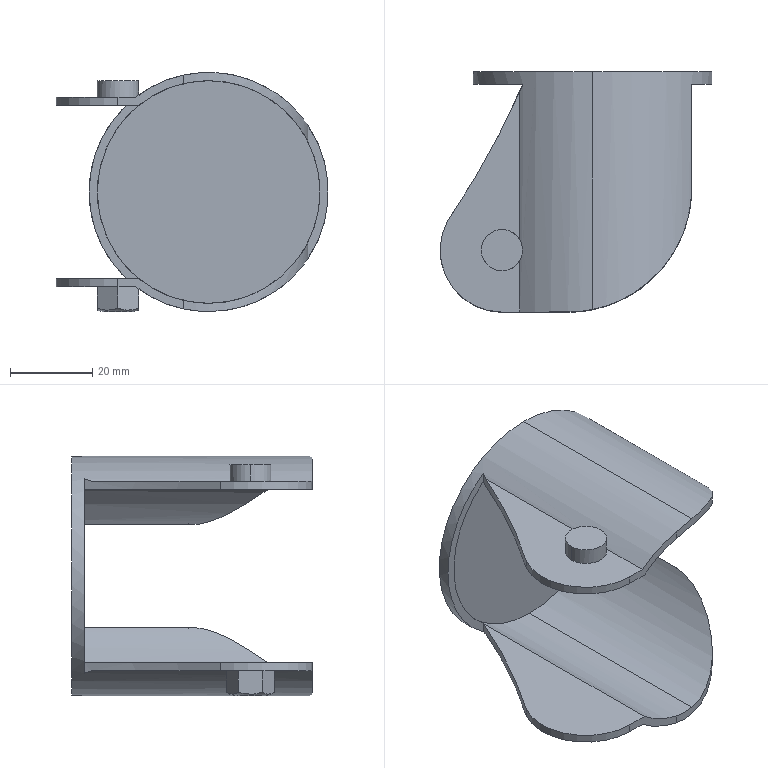Part | SolidWorks | features RefAxis 15, ICE 6, 3DProfileFeature 5, Revolution 2 | 1 solid | 36 faces | box 66 x 58.3 x 58 mm | volume 18491 mm3 | plane 20 | cylinder 14 | torus 2 | commonest cylinder face diameters 10 x2 12 x2 30 x2 54 x2 58 x2 60 x2
STEP:
#1=CARTESIAN_POINT('',(-17.,-56.613,-28.187));
#2=VERTEX_POINT('',#1);
#3=CARTESIAN_POINT('',(-17.,-59.5,-28.653));
#4=VERTEX_POINT('',#3);
#5=CARTESIAN_POINT('',(-17.,-56.613,-28.187));
#6=CARTESIAN_POINT('',(-17.,-56.842,-28.275));
#7=CARTESIAN_POINT('',(-17.,-57.08,-28.349));
#8=CARTESIAN_POINT('',(-17.,-57.557,-28.468));
#9=CARTESIAN_POINT('',(-17.,-57.797,-28.514));
#10=CARTESIAN_POINT('',(-17.,-58.521,-28.621));
#11=CARTESIAN_POINT('',(-17.,-59.009,-28.653));
#12=CARTESIAN_POINT('',(-17.,-59.5,-28.653));
#13=B_SPLINE_CURVE_WITH_KNOTS('',3,(#5,#6,#7,#8,#9,#10,#11,#12),.UNSPECIFIED.,.F.,.F.,(4,2,2,4),(0.007838,0.008573,0.009308,0.01078),.UNSPECIFIED.);
#14=EDGE_CURVE('',#2,#4,#13,.T.);
#15=ORIENTED_EDGE('',*,*,#14,.T.);
#16=CARTESIAN_POINT('',(-18.324,-59.5,-29.));
#17=VERTEX_POINT('',#16);
#18=CARTESIAN_POINT('',(-18.662,-59.5,-25.014));
#19=DIRECTION('',(0.,1.,0.));
#20=DIRECTION('',(-1.,0.,0.));
#21=AXIS2_PLACEMENT_3D('',#18,#19,#20);
#22=CIRCLE('',#21,4.);
#23=EDGE_CURVE('',#4,#17,#22,.T.);
#24=ORIENTED_EDGE('',*,*,#23,.T.);
#25=CARTESIAN_POINT('',(-25.676,-59.5,-29.));
#26=VERTEX_POINT('',#25);
#27=CARTESIAN_POINT('',(-22.,-59.5,-29.));
#28=DIRECTION('',(0.,0.,-1.));
#29=DIRECTION('',(-1.,0.,0.));
#30=AXIS2_PLACEMENT_3D('',#27,#28,#29);
#31=CIRCLE('',#30,3.676);
#32=EDGE_CURVE('',#26,#17,#31,.T.);
#33=ORIENTED_EDGE('',*,*,#32,.F.);
#34=CARTESIAN_POINT('',(-27.,-59.5,-28.653));
#35=VERTEX_POINT('',#34);
#36=CARTESIAN_POINT('',(-25.338,-59.5,-25.014));
#37=DIRECTION('',(0.,-1.,0.));
#38=DIRECTION('',(0.,0.,-1.));
#39=AXIS2_PLACEMENT_3D('',#36,#37,#38);
#40=CIRCLE('',#39,4.);
#41=EDGE_CURVE('',#35,#26,#40,.T.);
#42=ORIENTED_EDGE('',*,*,#41,.F.);
#43=CARTESIAN_POINT('',(-27.,-56.613,-28.187));
#44=VERTEX_POINT('',#43);
#45=CARTESIAN_POINT('',(-27.,-59.5,-28.653));
#46=CARTESIAN_POINT('',(-27.,-59.007,-28.653));
#47=CARTESIAN_POINT('',(-27.,-58.515,-28.621));
#48=CARTESIAN_POINT('',(-27.,-57.55,-28.477));
#49=CARTESIAN_POINT('',(-27.,-57.076,-28.365));
#50=CARTESIAN_POINT('',(-27.,-56.613,-28.187));
#51=B_SPLINE_CURVE_WITH_KNOTS('',3,(#45,#46,#47,#48,#49,#50),.UNSPECIFIED.,.F.,.F.,(4,2,4),(0.01078,0.01225,0.01373),.UNSPECIFIED.);
#52=EDGE_CURVE('',#35,#44,#51,.T.);
#53=ORIENTED_EDGE('',*,*,#52,.T.);
#54=CARTESIAN_POINT('',(-22.,-53.726,-28.187));
#55=VERTEX_POINT('',#54);
#56=CARTESIAN_POINT('',(-27.,-56.613,-28.187));
#57=CARTESIAN_POINT('',(-26.6,-56.382,-28.365));
#58=CARTESIAN_POINT('',(-26.188,-56.145,-28.477));
#59=CARTESIAN_POINT('',(-25.352,-55.662,-28.621));
#60=CARTESIAN_POINT('',(-24.924,-55.415,-28.653));
#61=CARTESIAN_POINT('',(-24.077,-54.926,-28.653));
#62=CARTESIAN_POINT('',(-23.656,-54.682,-28.622));
#63=CARTESIAN_POINT('',(-22.819,-54.199,-28.479));
#64=CARTESIAN_POINT('',(-22.4,-53.957,-28.365));
#65=CARTESIAN_POINT('',(-22.,-53.726,-28.187));
#66=B_SPLINE_CURVE_WITH_KNOTS('',3,(#56,#57,#58,#59,#60,#61,#62,#63,#64,#65),.UNSPECIFIED.,.F.,.F.,(4,2,2,2,4),(0.000000244,0.001463,0.002926,0.00439,0.005853),.UNSPECIFIED.);
#67=EDGE_CURVE('',#44,#55,#66,.T.);
#68=ORIENTED_EDGE('',*,*,#67,.T.);
#69=CARTESIAN_POINT('',(-22.,-53.726,-28.187));
#70=CARTESIAN_POINT('',(-21.6,-53.958,-28.365));
#71=CARTESIAN_POINT('',(-21.188,-54.195,-28.477));
#72=CARTESIAN_POINT('',(-20.352,-54.678,-28.621));
#73=CARTESIAN_POINT('',(-19.924,-54.925,-28.653));
#74=CARTESIAN_POINT('',(-19.077,-55.414,-28.653));
#75=CARTESIAN_POINT('',(-18.656,-55.657,-28.622));
#76=CARTESIAN_POINT('',(-17.819,-56.141,-28.479));
#77=CARTESIAN_POINT('',(-17.4,-56.382,-28.365));
#78=CARTESIAN_POINT('',(-17.,-56.613,-28.187));
#79=B_SPLINE_CURVE_WITH_KNOTS('',3,(#69,#70,#71,#72,#73,#74,#75,#76,#77,#78),.UNSPECIFIED.,.F.,.F.,(4,2,2,2,4),(0.000000244,0.001463,0.002926,0.00439,0.005853),.UNSPECIFIED.);
#80=EDGE_CURVE('',#55,#2,#79,.T.);
#81=ORIENTED_EDGE('',*,*,#80,.T.);
#82=EDGE_LOOP('',(#15,#24,#33,#42,#53,#68,#81));
#83=FACE_OUTER_BOUND('',#82,.T.);
#84=CARTESIAN_POINT('',(-22.,-59.5,-25.014));
#85=DIRECTION('',(0.,0.,-1.));
#86=DIRECTION('',(-1.,0.,0.));
#87=AXIS2_PLACEMENT_3D('',#84,#85,#86);
#88=TOROIDAL_SURFACE('',#87,3.338,4.);
#89=ADVANCED_FACE('',(#83),#88,.T.);
#90=CARTESIAN_POINT('',(-17.664,-55.353,-23.));
#91=VERTEX_POINT('',#90);
#92=CARTESIAN_POINT('',(-16.,-59.5,-24.187));
#93=VERTEX_POINT('',#92);
#94=CARTESIAN_POINT('',(-17.664,-55.353,-23.));
#95=CARTESIAN_POINT('',(-17.419,-55.609,-23.188));
#96=CARTESIAN_POINT('',(-17.194,-55.89,-23.355));
#97=CARTESIAN_POINT('',(-16.787,-56.506,-23.649));
#98=CARTESIAN_POINT('',(-16.605,-56.846,-23.776));
#99=CARTESIAN_POINT('',(-16.311,-57.555,-23.979));
#100=CARTESIAN_POINT('',(-16.197,-57.926,-24.056));
#101=CARTESIAN_POINT('',(-16.079,-58.509,-24.134));
#102=CARTESIAN_POINT('',(-16.049,-58.708,-24.154));
#103=CARTESIAN_POINT('',(-16.01,-59.104,-24.18));
#104=CARTESIAN_POINT('',(-16.,-59.302,-24.187));
#105=CARTESIAN_POINT('',(-16.,-59.5,-24.187));
#106=B_SPLINE_CURVE_WITH_KNOTS('',3,(#94,#95,#96,#97,#98,#99,#100,#101,#102,#103,#104,#105),.UNSPECIFIED.,.F.,.F.,(4,2,2,2,2,4),(0.01597,0.01715,0.01833,0.01951,0.0201,0.02069),.UNSPECIFIED.);
#107=EDGE_CURVE('',#91,#93,#106,.T.);
#108=ORIENTED_EDGE('',*,*,#107,.T.);
#109=CARTESIAN_POINT('',(-16.,-59.5,-23.));
#110=VERTEX_POINT('',#109);
#111=CARTESIAN_POINT('',(-16.,-59.5,-33.));
#112=DIRECTION('',(0.,0.,1.));
#113=VECTOR('',#112,1000.);
#114=LINE('',#111,#113);
#115=EDGE_CURVE('',#93,#110,#114,.T.);
#116=ORIENTED_EDGE('',*,*,#115,.T.);
#117=CARTESIAN_POINT('',(-22.,-59.5,-23.));
#118=DIRECTION('',(0.,0.,1.));
#119=DIRECTION('',(1.,0.,0.));
#120=AXIS2_PLACEMENT_3D('',#117,#118,#119);
#121=CIRCLE('',#120,6.);
#122=EDGE_CURVE('',#110,#91,#121,.T.);
#123=ORIENTED_EDGE('',*,*,#122,.T.);
#124=EDGE_LOOP('',(#108,#116,#123));
#125=FACE_OUTER_BOUND('',#124,.T.);
#126=CARTESIAN_POINT('',(-22.,-59.5,-33.));
#127=DIRECTION('',(0.,0.,1.));
#128=DIRECTION('',(1.,0.,0.));
#129=AXIS2_PLACEMENT_3D('',#126,#127,#128);
#130=CYLINDRICAL_SURFACE('',#129,6.);
#131=ADVANCED_FACE('',(#125),#130,.F.);
#132=CARTESIAN_POINT('',(-17.,-59.5,27.));
#133=VERTEX_POINT('',#132);
#134=CARTESIAN_POINT('',(-27.,-59.5,27.));
#135=VERTEX_POINT('',#134);
#136=CARTESIAN_POINT('',(-22.,-59.5,27.));
#137=DIRECTION('',(0.,0.,1.));
#138=DIRECTION('',(1.,0.,0.));
#139=AXIS2_PLACEMENT_3D('',#136,#137,#138);
#140=CIRCLE('',#139,5.);
#141=EDGE_CURVE('',#133,#135,#140,.T.);
#142=ORIENTED_EDGE('',*,*,#141,.F.);
#143=CARTESIAN_POINT('',(-17.,-59.5,23.495));
#144=VERTEX_POINT('',#143);
#145=CARTESIAN_POINT('',(-17.,-59.5,27.));
#146=DIRECTION('',(0.,0.,-1.));
#147=VECTOR('',#146,1000.);
#148=LINE('',#145,#147);
#149=EDGE_CURVE('',#133,#144,#148,.T.);
#150=ORIENTED_EDGE('',*,*,#149,.T.);
#151=CARTESIAN_POINT('',(-17.664,-57.011,23.));
#152=VERTEX_POINT('',#151);
#153=CARTESIAN_POINT('',(-17.664,-57.011,23.));
#154=CARTESIAN_POINT('',(-17.455,-57.374,23.16));
#155=CARTESIAN_POINT('',(-17.29,-57.767,23.283));
#156=CARTESIAN_POINT('',(-17.117,-58.403,23.41));
#157=CARTESIAN_POINT('',(-17.073,-58.62,23.442));
#158=CARTESIAN_POINT('',(-17.015,-59.057,23.484));
#159=CARTESIAN_POINT('',(-17.,-59.277,23.495));
#160=CARTESIAN_POINT('',(-17.,-59.5,23.495));
#161=B_SPLINE_CURVE_WITH_KNOTS('',3,(#153,#154,#155,#156,#157,#158,#159,#160),.UNSPECIFIED.,.F.,.F.,(4,2,2,4),(0.,0.001329,0.001993,0.002657),.UNSPECIFIED.);
#162=EDGE_CURVE('',#152,#144,#161,.T.);
#163=ORIENTED_EDGE('',*,*,#162,.F.);
#164=CARTESIAN_POINT('',(-27.,-59.5,23.));
#165=VERTEX_POINT('',#164);
#166=CARTESIAN_POINT('',(-22.,-59.5,23.));
#167=DIRECTION('',(0.,0.,1.));
#168=DIRECTION('',(1.,0.,0.));
#169=AXIS2_PLACEMENT_3D('',#166,#167,#168);
#170=CIRCLE('',#169,5.);
#171=EDGE_CURVE('',#152,#165,#170,.T.);
#172=ORIENTED_EDGE('',*,*,#171,.T.);
#173=CARTESIAN_POINT('',(-27.,-59.5,27.));
#174=DIRECTION('',(0.,0.,-1.));
#175=VECTOR('',#174,1000.);
#176=LINE('',#173,#175);
#177=EDGE_CURVE('',#135,#165,#176,.T.);
#178=ORIENTED_EDGE('',*,*,#177,.F.);
#179=EDGE_LOOP('',(#142,#150,#163,#172,#178));
#180=FACE_OUTER_BOUND('',#179,.T.);
#181=CARTESIAN_POINT('',(-22.,-59.5,27.));
#182=DIRECTION('',(0.,0.,-1.));
#183=DIRECTION('',(-1.,0.,0.));
#184=AXIS2_PLACEMENT_3D('',#181,#182,#183);
#185=CYLINDRICAL_SURFACE('',#184,5.);
#186=ADVANCED_FACE('',(#180),#185,.T.);
#187=CARTESIAN_POINT('',(0.,-73.894,-27.));
#188=VERTEX_POINT('',#187);
#189=CARTESIAN_POINT('',(-6.,-74.5,-26.325));
#190=VERTEX_POINT('',#189);
#191=CARTESIAN_POINT('',(0.,-73.894,-27.));
#192=CARTESIAN_POINT('',(-2.,-74.302,-27.));
#193=CARTESIAN_POINT('',(-4.001,-74.5,-26.781));
#194=CARTESIAN_POINT('',(-6.,-74.5,-26.325));
#195=B_SPLINE_CURVE_WITH_KNOTS('',3,(#191,#192,#193,#194),.UNSPECIFIED.,.F.,.F.,(4,4),(0.04396,0.05001),.UNSPECIFIED.);
#196=EDGE_CURVE('',#188,#190,#195,.T.);
#197=ORIENTED_EDGE('',*,*,#196,.F.);
#198=CARTESIAN_POINT('',(0.,-18.2,-27.));
#199=VERTEX_POINT('',#198);
#200=CARTESIAN_POINT('',(0.,-16.2,-27.));
#201=DIRECTION('',(0.,1.,0.));
#202=VECTOR('',#201,1000.);
#203=LINE('',#200,#202);
#204=EDGE_CURVE('',#188,#199,#203,.T.);
#205=ORIENTED_EDGE('',*,*,#204,.T.);
#206=CARTESIAN_POINT('',(0.,-18.2,27.));
#207=VERTEX_POINT('',#206);
#208=CARTESIAN_POINT('',(0.,-18.2,0.));
#209=DIRECTION('',(0.,1.,0.));
#210=DIRECTION('',(0.,0.,1.));
#211=AXIS2_PLACEMENT_3D('',#208,#209,#210);
#212=CIRCLE('',#211,27.);
#213=EDGE_CURVE('',#199,#207,#212,.T.);
#214=ORIENTED_EDGE('',*,*,#213,.T.);
#215=CARTESIAN_POINT('',(0.,-73.894,27.));
#216=VERTEX_POINT('',#215);
#217=CARTESIAN_POINT('',(0.,-16.2,27.));
#218=DIRECTION('',(0.,1.,0.));
#219=VECTOR('',#218,1000.);
#220=LINE('',#217,#219);
#221=EDGE_CURVE('',#216,#207,#220,.T.);
#222=ORIENTED_EDGE('',*,*,#221,.F.);
#223=CARTESIAN_POINT('',(-6.,-74.5,26.325));
#224=VERTEX_POINT('',#223);
#225=CARTESIAN_POINT('',(-6.,-74.5,26.325));
#226=CARTESIAN_POINT('',(-3.997,-74.5,26.781));
#227=CARTESIAN_POINT('',(-1.996,-74.301,27.));
#228=CARTESIAN_POINT('',(0.,-73.894,27.));
#229=B_SPLINE_CURVE_WITH_KNOTS('',3,(#225,#226,#227,#228),.UNSPECIFIED.,.F.,.F.,(4,4),(0.,0.006066),.UNSPECIFIED.);
#230=EDGE_CURVE('',#224,#216,#229,.T.);
#231=ORIENTED_EDGE('',*,*,#230,.F.);
#232=CARTESIAN_POINT('',(-16.971,-74.5,21.));
#233=VERTEX_POINT('',#232);
#234=CARTESIAN_POINT('',(0.,-74.5,0.));
#235=DIRECTION('',(0.,1.,0.));
#236=DIRECTION('',(0.,0.,1.));
#237=AXIS2_PLACEMENT_3D('',#234,#235,#236);
#238=CIRCLE('',#237,27.);
#239=EDGE_CURVE('',#233,#224,#238,.T.);
#240=ORIENTED_EDGE('',*,*,#239,.F.);
#241=CARTESIAN_POINT('',(-16.971,-19.329,21.));
#242=VERTEX_POINT('',#241);
#243=CARTESIAN_POINT('',(-16.971,-118.2,21.));
#244=DIRECTION('',(0.,1.,0.));
#245=VECTOR('',#244,1000.);
#246=LINE('',#243,#245);
#247=EDGE_CURVE('',#233,#242,#246,.T.);
#248=ORIENTED_EDGE('',*,*,#247,.T.);
#249=CARTESIAN_POINT('',(-16.916,-19.2,21.044));
#250=VERTEX_POINT('',#249);
#251=CARTESIAN_POINT('',(-16.916,-19.2,21.044));
#252=CARTESIAN_POINT('',(-16.934,-19.243,21.03));
#253=CARTESIAN_POINT('',(-16.952,-19.286,21.015));
#254=CARTESIAN_POINT('',(-16.971,-19.329,21.));
#255=B_SPLINE_CURVE_WITH_KNOTS('',3,(#251,#252,#253,#254),.UNSPECIFIED.,.F.,.F.,(4,4),(0.,0.0001456),.UNSPECIFIED.);
#256=EDGE_CURVE('',#250,#242,#255,.T.);
#257=ORIENTED_EDGE('',*,*,#256,.F.);
#258=CARTESIAN_POINT('',(-16.916,-19.2,-21.044));
#259=VERTEX_POINT('',#258);
#260=CARTESIAN_POINT('',(0.,-19.2,0.));
#261=DIRECTION('',(0.,1.,0.));
#262=DIRECTION('',(0.,0.,1.));
#263=AXIS2_PLACEMENT_3D('',#260,#261,#262);
#264=CIRCLE('',#263,27.);
#265=EDGE_CURVE('',#259,#250,#264,.T.);
#266=ORIENTED_EDGE('',*,*,#265,.F.);
#267=CARTESIAN_POINT('',(-16.971,-19.329,-21.));
#268=VERTEX_POINT('',#267);
#269=CARTESIAN_POINT('',(-16.971,-19.329,-21.));
#270=CARTESIAN_POINT('',(-16.952,-19.286,-21.015));
#271=CARTESIAN_POINT('',(-16.934,-19.243,-21.03));
#272=CARTESIAN_POINT('',(-16.916,-19.2,-21.044));
#273=B_SPLINE_CURVE_WITH_KNOTS('',3,(#269,#270,#271,#272),.UNSPECIFIED.,.F.,.F.,(4,4),(0.06533,0.06547),.UNSPECIFIED.);
#274=EDGE_CURVE('',#268,#259,#273,.T.);
#275=ORIENTED_EDGE('',*,*,#274,.F.);
#276=CARTESIAN_POINT('',(-16.971,-74.5,-21.));
#277=VERTEX_POINT('',#276);
#278=CARTESIAN_POINT('',(-16.971,-118.2,-21.));
#279=DIRECTION('',(0.,-1.,0.));
#280=VECTOR('',#279,1000.);
#281=LINE('',#278,#280);
#282=EDGE_CURVE('',#268,#277,#281,.T.);
#283=ORIENTED_EDGE('',*,*,#282,.T.);
#284=CARTESIAN_POINT('',(0.,-74.5,0.));
#285=DIRECTION('',(0.,1.,0.));
#286=DIRECTION('',(0.,0.,1.));
#287=AXIS2_PLACEMENT_3D('',#284,#285,#286);
#288=CIRCLE('',#287,27.);
#289=EDGE_CURVE('',#190,#277,#288,.T.);
#290=ORIENTED_EDGE('',*,*,#289,.F.);
#291=EDGE_LOOP('',(#197,#205,#214,#222,#231,#240,#248,#257,#266,#275,#283,#290));
#292=FACE_OUTER_BOUND('',#291,.T.);
#293=CARTESIAN_POINT('',(0.,-16.2,0.));
#294=DIRECTION('',(0.,1.,0.));
#295=DIRECTION('',(0.,0.,1.));
#296=AXIS2_PLACEMENT_3D('',#293,#294,#295);
#297=CYLINDRICAL_SURFACE('',#296,27.);
#298=ADVANCED_FACE('',(#292),#297,.F.);
#299=CARTESIAN_POINT('',(0.,-73.894,-29.));
#300=VERTEX_POINT('',#299);
#301=CARTESIAN_POINT('',(24.,-44.5,-16.279));
#302=VERTEX_POINT('',#301);
#303=CARTESIAN_POINT('',(0.,-73.894,-29.));
#304=CARTESIAN_POINT('',(0.8866,-73.713,-29.));
#305=CARTESIAN_POINT('',(1.776,-73.489,-28.959));
#306=CARTESIAN_POINT('',(3.506,-72.968,-28.8));
#307=CARTESIAN_POINT('',(4.35,-72.672,-28.684));
#308=CARTESIAN_POINT('',(6.,-72.01,-28.385));
#309=CARTESIAN_POINT('',(6.806,-71.644,-28.202));
#310=CARTESIAN_POINT('',(7.986,-71.044,-27.882));
#311=CARTESIAN_POINT('',(8.376,-70.835,-27.767));
#312=CARTESIAN_POINT('',(9.139,-70.403,-27.525));
#313=CARTESIAN_POINT('',(9.513,-70.181,-27.398));
#314=CARTESIAN_POINT('',(11.345,-69.039,-26.734));
#315=CARTESIAN_POINT('',(12.693,-68.024,-26.113));
#316=CARTESIAN_POINT('',(14.564,-66.359,-25.088));
#317=CARTESIAN_POINT('',(15.164,-65.779,-24.729));
#318=CARTESIAN_POINT('',(16.308,-64.576,-23.99));
#319=CARTESIAN_POINT('',(16.849,-63.958,-23.612));
#320=CARTESIAN_POINT('',(18.383,-62.054,-22.466));
#321=CARTESIAN_POINT('',(19.29,-60.719,-21.682));
#322=CARTESIAN_POINT('',(20.493,-58.599,-20.527));
#323=CARTESIAN_POINT('',(20.867,-57.874,-20.145));
#324=CARTESIAN_POINT('',(21.562,-56.376,-19.4));
#325=CARTESIAN_POINT('',(21.882,-55.603,-19.036));
#326=CARTESIAN_POINT('',(22.747,-53.242,-18.01));
#327=CARTESIAN_POINT('',(23.201,-51.602,-17.407));
#328=CARTESIAN_POINT('',(23.596,-49.428,-16.86));
#329=CARTESIAN_POINT('',(23.666,-48.987,-16.761));
#330=CARTESIAN_POINT('',(23.786,-48.103,-16.59));
#331=CARTESIAN_POINT('',(23.837,-47.658,-16.517));
#332=CARTESIAN_POINT('',(23.958,-46.318,-16.341));
#333=CARTESIAN_POINT('',(24.,-45.414,-16.279));
#334=CARTESIAN_POINT('',(24.,-44.5,-16.279));
#335=B_SPLINE_CURVE_WITH_KNOTS('',3,(#303,#304,#305,#306,#307,#308,#309,#310,#311,#312,#313,#314,#315,#316,#317,#318,#319,#320,#321,#322,#323,#324,#325,#326,#327,#328,#329,#330,#331,#332,#333,#334),.UNSPECIFIED.,.F.,.F.,(4,2,2,2,2,2,2,2,2,2,2,2,2,2,2,4),(0.00606,0.008758,0.01146,0.01415,0.0155,0.01685,0.02225,0.02495,0.02765,0.03304,0.03574,0.03844,0.04384,0.04518,0.04653,0.04923),.UNSPECIFIED.);
#336=EDGE_CURVE('',#300,#302,#335,.T.);
#337=ORIENTED_EDGE('',*,*,#336,.F.);
#338=CARTESIAN_POINT('',(0.,-16.2,-29.));
#339=VERTEX_POINT('',#338);
#340=CARTESIAN_POINT('',(0.,-16.2,-29.));
#341=DIRECTION('',(0.,1.,0.));
#342=VECTOR('',#341,1000.);
#343=LINE('',#340,#342);
#344=EDGE_CURVE('',#300,#339,#343,.T.);
#345=ORIENTED_EDGE('',*,*,#344,.T.);
#346=CARTESIAN_POINT('',(0.,-16.2,29.));
#347=VERTEX_POINT('',#346);
#348=CARTESIAN_POINT('',(0.,-16.2,0.));
#349=DIRECTION('',(0.,1.,0.));
#350=DIRECTION('',(0.,0.,1.));
#351=AXIS2_PLACEMENT_3D('',#348,#349,#350);
#352=CIRCLE('',#351,29.);
#353=EDGE_CURVE('',#347,#339,#352,.T.);
#354=ORIENTED_EDGE('',*,*,#353,.F.);
#355=CARTESIAN_POINT('',(0.,-73.894,29.));
#356=VERTEX_POINT('',#355);
#357=CARTESIAN_POINT('',(0.,-16.2,29.));
#358=DIRECTION('',(0.,1.,0.));
#359=VECTOR('',#358,1000.);
#360=LINE('',#357,#359);
#361=EDGE_CURVE('',#356,#347,#360,.T.);
#362=ORIENTED_EDGE('',*,*,#361,.F.);
#363=CARTESIAN_POINT('',(24.,-44.5,16.279));
#364=VERTEX_POINT('',#363);
#365=CARTESIAN_POINT('',(24.,-44.5,16.279));
#366=CARTESIAN_POINT('',(24.,-46.333,16.279));
#367=CARTESIAN_POINT('',(23.834,-48.111,16.53));
#368=CARTESIAN_POINT('',(23.442,-50.278,17.073));
#369=CARTESIAN_POINT('',(23.354,-50.709,17.194));
#370=CARTESIAN_POINT('',(23.16,-51.562,17.454));
#371=CARTESIAN_POINT('',(23.055,-51.982,17.592));
#372=CARTESIAN_POINT('',(22.717,-53.222,18.03));
#373=CARTESIAN_POINT('',(22.46,-54.025,18.351));
#374=CARTESIAN_POINT('',(21.887,-55.592,19.031));
#375=CARTESIAN_POINT('',(21.57,-56.355,19.39));
#376=CARTESIAN_POINT('',(20.878,-57.85,20.133));
#377=CARTESIAN_POINT('',(20.502,-58.583,20.518));
#378=CARTESIAN_POINT('',(19.287,-60.725,21.686));
#379=CARTESIAN_POINT('',(18.375,-62.065,22.472));
#380=CARTESIAN_POINT('',(16.335,-64.595,23.996));
#381=CARTESIAN_POINT('',(15.207,-65.786,24.735));
#382=CARTESIAN_POINT('',(13.639,-67.182,25.595));
#383=CARTESIAN_POINT('',(13.317,-67.458,25.764));
#384=CARTESIAN_POINT('',(12.66,-67.994,26.093));
#385=CARTESIAN_POINT('',(12.326,-68.256,26.253));
#386=CARTESIAN_POINT('',(11.305,-69.021,26.716));
#387=CARTESIAN_POINT('',(10.6,-69.504,27.005));
#388=CARTESIAN_POINT('',(9.138,-70.415,27.534));
#389=CARTESIAN_POINT('',(8.381,-70.843,27.774));
#390=CARTESIAN_POINT('',(6.812,-71.641,28.2));
#391=CARTESIAN_POINT('',(5.993,-72.013,28.386));
#392=CARTESIAN_POINT('',(3.502,-73.012,28.837));
#393=CARTESIAN_POINT('',(1.782,-73.53,29.));
#394=CARTESIAN_POINT('',(0.,-73.894,29.));
#395=B_SPLINE_CURVE_WITH_KNOTS('',3,(#365,#366,#367,#368,#369,#370,#371,#372,#373,#374,#375,#376,#377,#378,#379,#380,#381,#382,#383,#384,#385,#386,#387,#388,#389,#390,#391,#392,#393,#394),.UNSPECIFIED.,.F.,.F.,(4,2,2,2,2,2,2,2,2,2,2,2,2,2,4),(0.,0.005407,0.006759,0.008111,0.01081,0.01352,0.01622,0.02163,0.02704,0.02839,0.02974,0.03244,0.03515,0.03785,0.04326),.UNSPECIFIED.);
#396=EDGE_CURVE('',#364,#356,#395,.T.);
#397=ORIENTED_EDGE('',*,*,#396,.F.);
#398=CARTESIAN_POINT('',(24.,-19.2,16.279));
#399=VERTEX_POINT('',#398);
#400=CARTESIAN_POINT('',(24.,-16.2,16.279));
#401=DIRECTION('',(0.,-1.,0.));
#402=VECTOR('',#401,1000.);
#403=LINE('',#400,#402);
#404=EDGE_CURVE('',#399,#364,#403,.T.);
#405=ORIENTED_EDGE('',*,*,#404,.F.);
#406=CARTESIAN_POINT('',(24.,-19.2,-16.279));
#407=VERTEX_POINT('',#406);
#408=CARTESIAN_POINT('',(0.,-19.2,0.));
#409=DIRECTION('',(0.,-1.,0.));
#410=DIRECTION('',(-1.,0.,0.));
#411=AXIS2_PLACEMENT_3D('',#408,#409,#410);
#412=CIRCLE('',#411,29.);
#413=EDGE_CURVE('',#407,#399,#412,.T.);
#414=ORIENTED_EDGE('',*,*,#413,.F.);
#415=CARTESIAN_POINT('',(24.,-16.2,-16.279));
#416=DIRECTION('',(0.,1.,0.));
#417=VECTOR('',#416,1000.);
#418=LINE('',#415,#417);
#419=EDGE_CURVE('',#302,#407,#418,.T.);
#420=ORIENTED_EDGE('',*,*,#419,.F.);
#421=EDGE_LOOP('',(#337,#345,#354,#362,#397,#405,#414,#420));
#422=FACE_OUTER_BOUND('',#421,.T.);
#423=CARTESIAN_POINT('',(0.,-16.2,0.));
#424=DIRECTION('',(0.,1.,0.));
#425=DIRECTION('',(0.,0.,1.));
#426=AXIS2_PLACEMENT_3D('',#423,#424,#425);
#427=CYLINDRICAL_SURFACE('',#426,29.);
#428=ADVANCED_FACE('',(#422),#427,.T.);
#429=ORIENTED_EDGE('',*,*,#344,.F.);
#430=CARTESIAN_POINT('',(-6.,-74.5,-28.373));
#431=VERTEX_POINT('',#430);
#432=CARTESIAN_POINT('',(-6.,-74.5,-28.373));
#433=CARTESIAN_POINT('',(-3.992,-74.5,-28.797));
#434=CARTESIAN_POINT('',(-1.991,-74.3,-29.));
#435=CARTESIAN_POINT('',(0.,-73.894,-29.));
#436=B_SPLINE_CURVE_WITH_KNOTS('',3,(#432,#433,#434,#435),.UNSPECIFIED.,.F.,.F.,(4,4),(0.,0.00606),.UNSPECIFIED.);
#437=EDGE_CURVE('',#431,#300,#436,.T.);
#438=ORIENTED_EDGE('',*,*,#437,.F.);
#439=CARTESIAN_POINT('',(-17.664,-74.5,-23.));
#440=VERTEX_POINT('',#439);
#441=CARTESIAN_POINT('',(0.,-74.5,0.));
#442=DIRECTION('',(0.,-1.,0.));
#443=DIRECTION('',(0.,0.,1.));
#444=AXIS2_PLACEMENT_3D('',#441,#442,#443);
#445=CIRCLE('',#444,29.);
#446=EDGE_CURVE('',#440,#431,#445,.T.);
#447=ORIENTED_EDGE('',*,*,#446,.F.);
#448=CARTESIAN_POINT('',(-17.664,-63.647,-23.));
#449=VERTEX_POINT('',#448);
#450=CARTESIAN_POINT('',(-17.664,-16.2,-23.));
#451=DIRECTION('',(0.,-1.,0.));
#452=VECTOR('',#451,1000.);
#453=LINE('',#450,#452);
#454=EDGE_CURVE('',#449,#440,#453,.T.);
#455=ORIENTED_EDGE('',*,*,#454,.F.);
#456=CARTESIAN_POINT('',(-16.,-59.5,-24.187));
#457=CARTESIAN_POINT('',(-16.,-59.698,-24.187));
#458=CARTESIAN_POINT('',(-16.01,-59.896,-24.18));
#459=CARTESIAN_POINT('',(-16.049,-60.292,-24.154));
#460=CARTESIAN_POINT('',(-16.079,-60.49,-24.134));
#461=CARTESIAN_POINT('',(-16.196,-61.07,-24.056));
#462=CARTESIAN_POINT('',(-16.31,-61.442,-23.98));
#463=CARTESIAN_POINT('',(-16.606,-62.157,-23.775));
#464=CARTESIAN_POINT('',(-16.786,-62.491,-23.65));
#465=CARTESIAN_POINT('',(-17.191,-63.107,-23.356));
#466=CARTESIAN_POINT('',(-17.421,-63.393,-23.186));
#467=CARTESIAN_POINT('',(-17.664,-63.647,-23.));
#468=B_SPLINE_CURVE_WITH_KNOTS('',3,(#456,#457,#458,#459,#460,#461,#462,#463,#464,#465,#466,#467),.UNSPECIFIED.,.F.,.F.,(4,2,2,2,2,4),(0.02069,0.02128,0.02186,0.02304,0.02422,0.02539),.UNSPECIFIED.);
#469=EDGE_CURVE('',#93,#449,#468,.T.);
#470=ORIENTED_EDGE('',*,*,#469,.F.);
#471=ORIENTED_EDGE('',*,*,#107,.F.);
#472=CARTESIAN_POINT('',(-17.664,-20.929,-23.));
#473=VERTEX_POINT('',#472);
#474=CARTESIAN_POINT('',(-17.664,-16.2,-23.));
#475=DIRECTION('',(0.,-1.,0.));
#476=VECTOR('',#475,1000.);
#477=LINE('',#474,#476);
#478=EDGE_CURVE('',#473,#91,#477,.T.);
#479=ORIENTED_EDGE('',*,*,#478,.F.);
#480=CARTESIAN_POINT('',(-16.916,-19.2,-23.555));
#481=VERTEX_POINT('',#480);
#482=CARTESIAN_POINT('',(-16.916,-19.2,-23.555));
#483=CARTESIAN_POINT('',(-17.163,-19.781,-23.378));
#484=CARTESIAN_POINT('',(-17.413,-20.357,-23.193));
#485=CARTESIAN_POINT('',(-17.664,-20.929,-23.));
#486=B_SPLINE_CURVE_WITH_KNOTS('',3,(#482,#483,#484,#485),.UNSPECIFIED.,.F.,.F.,(4,4),(0.,0.001942),.UNSPECIFIED.);
#487=EDGE_CURVE('',#481,#473,#486,.T.);
#488=ORIENTED_EDGE('',*,*,#487,.F.);
#489=CARTESIAN_POINT('',(-16.916,-19.2,23.555));
#490=VERTEX_POINT('',#489);
#491=CARTESIAN_POINT('',(0.,-19.2,0.));
#492=DIRECTION('',(0.,-1.,0.));
#493=DIRECTION('',(0.,0.,1.));
#494=AXIS2_PLACEMENT_3D('',#491,#492,#493);
#495=CIRCLE('',#494,29.);
#496=EDGE_CURVE('',#490,#481,#495,.T.);
#497=ORIENTED_EDGE('',*,*,#496,.F.);
#498=CARTESIAN_POINT('',(-17.664,-20.929,23.));
#499=VERTEX_POINT('',#498);
#500=CARTESIAN_POINT('',(-17.664,-20.929,23.));
#501=CARTESIAN_POINT('',(-17.412,-20.356,23.193));
#502=CARTESIAN_POINT('',(-17.163,-19.78,23.378));
#503=CARTESIAN_POINT('',(-16.916,-19.2,23.555));
#504=B_SPLINE_CURVE_WITH_KNOTS('',3,(#500,#501,#502,#503),.UNSPECIFIED.,.F.,.F.,(4,4),(0.0729,0.07483),.UNSPECIFIED.);
#505=EDGE_CURVE('',#499,#490,#504,.T.);
#506=ORIENTED_EDGE('',*,*,#505,.F.);
#507=CARTESIAN_POINT('',(-17.664,-16.2,23.));
#508=DIRECTION('',(0.,1.,0.));
#509=VECTOR('',#508,1000.);
#510=LINE('',#507,#509);
#511=EDGE_CURVE('',#152,#499,#510,.T.);
#512=ORIENTED_EDGE('',*,*,#511,.F.);
#513=ORIENTED_EDGE('',*,*,#162,.T.);
#514=CARTESIAN_POINT('',(-17.664,-61.989,23.));
#515=VERTEX_POINT('',#514);
#516=CARTESIAN_POINT('',(-17.,-59.5,23.495));
#517=CARTESIAN_POINT('',(-17.,-59.722,23.495));
#518=CARTESIAN_POINT('',(-17.015,-59.946,23.484));
#519=CARTESIAN_POINT('',(-17.074,-60.383,23.441));
#520=CARTESIAN_POINT('',(-17.117,-60.597,23.41));
#521=CARTESIAN_POINT('',(-17.231,-61.018,23.326));
#522=CARTESIAN_POINT('',(-17.302,-61.224,23.273));
#523=CARTESIAN_POINT('',(-17.466,-61.619,23.151));
#524=CARTESIAN_POINT('',(-17.56,-61.808,23.08));
#525=CARTESIAN_POINT('',(-17.664,-61.989,23.));
#526=B_SPLINE_CURVE_WITH_KNOTS('',3,(#516,#517,#518,#519,#520,#521,#522,#523,#524,#525),.UNSPECIFIED.,.F.,.F.,(4,2,2,2,4),(0.002657,0.003319,0.003982,0.004644,0.005306),.UNSPECIFIED.);
#527=EDGE_CURVE('',#144,#515,#526,.T.);
#528=ORIENTED_EDGE('',*,*,#527,.T.);
#529=CARTESIAN_POINT('',(-17.664,-74.5,23.));
#530=VERTEX_POINT('',#529);
#531=CARTESIAN_POINT('',(-17.664,-16.2,23.));
#532=DIRECTION('',(0.,1.,0.));
#533=VECTOR('',#532,1000.);
#534=LINE('',#531,#533);
#535=EDGE_CURVE('',#530,#515,#534,.T.);
#536=ORIENTED_EDGE('',*,*,#535,.F.);
#537=CARTESIAN_POINT('',(-6.,-74.5,28.373));
#538=VERTEX_POINT('',#537);
#539=CARTESIAN_POINT('',(0.,-74.5,0.));
#540=DIRECTION('',(0.,-1.,0.));
#541=DIRECTION('',(0.,0.,1.));
#542=AXIS2_PLACEMENT_3D('',#539,#540,#541);
#543=CIRCLE('',#542,29.);
#544=EDGE_CURVE('',#538,#530,#543,.T.);
#545=ORIENTED_EDGE('',*,*,#544,.F.);
#546=CARTESIAN_POINT('',(0.,-73.894,29.));
#547=CARTESIAN_POINT('',(-0.4963,-73.995,29.));
#548=CARTESIAN_POINT('',(-0.999,-74.085,28.987));
#549=CARTESIAN_POINT('',(-2.002,-74.237,28.935));
#550=CARTESIAN_POINT('',(-2.503,-74.3,28.896));
#551=CARTESIAN_POINT('',(-4.004,-74.45,28.74));
#552=CARTESIAN_POINT('',(-5.003,-74.5,28.583));
#553=CARTESIAN_POINT('',(-6.,-74.5,28.373));
#554=B_SPLINE_CURVE_WITH_KNOTS('',3,(#546,#547,#548,#549,#550,#551,#552,#553),.UNSPECIFIED.,.F.,.F.,(4,2,2,4),(0.04326,0.04476,0.04627,0.04928),.UNSPECIFIED.);
#555=EDGE_CURVE('',#356,#538,#554,.T.);
#556=ORIENTED_EDGE('',*,*,#555,.F.);
#557=ORIENTED_EDGE('',*,*,#361,.T.);
#558=CARTESIAN_POINT('',(0.,-16.2,0.));
#559=DIRECTION('',(0.,1.,0.));
#560=DIRECTION('',(0.,0.,1.));
#561=AXIS2_PLACEMENT_3D('',#558,#559,#560);
#562=CIRCLE('',#561,29.);
#563=EDGE_CURVE('',#339,#347,#562,.T.);
#564=ORIENTED_EDGE('',*,*,#563,.F.);
#565=EDGE_LOOP('',(#429,#438,#447,#455,#470,#471,#479,#488,#497,#506,#512,#513,#528,#536,#545,#556,#557,#564));
#566=FACE_OUTER_BOUND('',#565,.T.);
#567=CARTESIAN_POINT('',(0.,-16.2,0.));
#568=DIRECTION('',(0.,1.,0.));
#569=DIRECTION('',(0.,0.,1.));
#570=AXIS2_PLACEMENT_3D('',#567,#568,#569);
#571=CYLINDRICAL_SURFACE('',#570,29.);
#572=ADVANCED_FACE('',(#566),#571,.T.);
#573=CARTESIAN_POINT('',(0.,-18.2,0.));
#574=DIRECTION('',(0.,1.,0.));
#575=DIRECTION('',(0.,0.,1.));
#576=AXIS2_PLACEMENT_3D('',#573,#574,#575);
#577=CIRCLE('',#576,27.);
#578=EDGE_CURVE('',#207,#199,#577,.T.);
#579=ORIENTED_EDGE('',*,*,#578,.F.);
#580=ORIENTED_EDGE('',*,*,#213,.F.);
#581=EDGE_LOOP('',(#579,#580));
#582=FACE_OUTER_BOUND('',#581,.T.);
#583=CARTESIAN_POINT('',(0.,-18.2,0.));
#584=DIRECTION('',(0.,-1.,0.));
#585=DIRECTION('',(0.,0.,-1.));
#586=AXIS2_PLACEMENT_3D('',#583,#584,#585);
#587=PLANE('',#586);
#588=ADVANCED_FACE('',(#582),#587,.T.);
#589=ORIENTED_EDGE('',*,*,#204,.F.);
#590=CARTESIAN_POINT('',(24.,-44.5,-12.369));
#591=VERTEX_POINT('',#590);
#592=CARTESIAN_POINT('',(24.,-44.5,-12.369));
#593=CARTESIAN_POINT('',(24.,-46.366,-12.369));
#594=CARTESIAN_POINT('',(23.829,-48.157,-12.713));
#595=CARTESIAN_POINT('',(23.351,-50.767,-13.558));
#596=CARTESIAN_POINT('',(23.158,-51.607,-13.888));
#597=CARTESIAN_POINT('',(22.713,-53.235,-14.605));
#598=CARTESIAN_POINT('',(22.46,-54.025,-14.994));
#599=CARTESIAN_POINT('',(21.895,-55.569,-15.806));
#600=CARTESIAN_POINT('',(21.584,-56.323,-16.231));
#601=CARTESIAN_POINT('',(20.902,-57.802,-17.1));
#602=CARTESIAN_POINT('',(20.533,-58.523,-17.543));
#603=CARTESIAN_POINT('',(19.35,-60.623,-18.867));
#604=CARTESIAN_POINT('',(18.458,-61.947,-19.749));
#605=CARTESIAN_POINT('',(16.95,-63.838,-21.027));
#606=CARTESIAN_POINT('',(16.419,-64.452,-21.446));
#607=CARTESIAN_POINT('',(15.575,-65.349,-22.058));
#608=CARTESIAN_POINT('',(15.286,-65.644,-22.259));
#609=CARTESIAN_POINT('',(14.692,-66.226,-22.656));
#610=CARTESIAN_POINT('',(14.386,-66.513,-22.851));
#611=CARTESIAN_POINT('',(12.822,-67.922,-23.807));
#612=CARTESIAN_POINT('',(11.469,-68.951,-24.494));
#613=CARTESIAN_POINT('',(9.265,-70.341,-25.373));
#614=CARTESIAN_POINT('',(8.501,-70.778,-25.64));
#615=CARTESIAN_POINT('',(7.306,-71.392,-25.996));
#616=CARTESIAN_POINT('',(6.9,-71.588,-26.107));
#617=CARTESIAN_POINT('',(6.082,-71.963,-26.309));
#618=CARTESIAN_POINT('',(5.669,-72.141,-26.402));
#619=CARTESIAN_POINT('',(4.414,-72.649,-26.65));
#620=CARTESIAN_POINT('',(3.558,-72.951,-26.779));
#621=CARTESIAN_POINT('',(2.246,-73.348,-26.91));
#622=CARTESIAN_POINT('',(1.803,-73.471,-26.943));
#623=CARTESIAN_POINT('',(0.9077,-73.698,-26.988));
#624=CARTESIAN_POINT('',(0.4534,-73.801,-27.));
#625=CARTESIAN_POINT('',(0.,-73.894,-27.));
#626=B_SPLINE_CURVE_WITH_KNOTS('',3,(#592,#593,#594,#595,#596,#597,#598,#599,#600,#601,#602,#603,#604,#605,#606,#607,#608,#609,#610,#611,#612,#613,#614,#615,#616,#617,#618,#619,#620,#621,#622,#623,#624,#625),.UNSPECIFIED.,.F.,.F.,(4,2,2,2,2,2,2,2,2,2,2,2,2,2,2,2,4),(0.,0.005494,0.008242,0.01099,0.01374,0.01648,0.02198,0.02472,0.0261,0.02747,0.03297,0.03571,0.03709,0.03846,0.04121,0.04258,0.04396),.UNSPECIFIED.);
#627=EDGE_CURVE('',#591,#188,#626,.T.);
#628=ORIENTED_EDGE('',*,*,#627,.F.);
#629=CARTESIAN_POINT('',(24.,-19.2,-12.369));
#630=VERTEX_POINT('',#629);
#631=CARTESIAN_POINT('',(24.,-16.2,-12.369));
#632=DIRECTION('',(0.,-1.,0.));
#633=VECTOR('',#632,1000.);
#634=LINE('',#631,#633);
#635=EDGE_CURVE('',#630,#591,#634,.T.);
#636=ORIENTED_EDGE('',*,*,#635,.F.);
#637=CARTESIAN_POINT('',(24.,-19.2,12.369));
#638=VERTEX_POINT('',#637);
#639=CARTESIAN_POINT('',(0.,-19.2,0.));
#640=DIRECTION('',(0.,1.,0.));
#641=DIRECTION('',(-1.,0.,0.));
#642=AXIS2_PLACEMENT_3D('',#639,#640,#641);
#643=CIRCLE('',#642,27.);
#644=EDGE_CURVE('',#638,#630,#643,.T.);
#645=ORIENTED_EDGE('',*,*,#644,.F.);
#646=CARTESIAN_POINT('',(24.,-44.5,12.369));
#647=VERTEX_POINT('',#646);
#648=CARTESIAN_POINT('',(24.,-16.2,12.369));
#649=DIRECTION('',(0.,1.,0.));
#650=VECTOR('',#649,1000.);
#651=LINE('',#648,#650);
#652=EDGE_CURVE('',#647,#638,#651,.T.);
#653=ORIENTED_EDGE('',*,*,#652,.F.);
#654=CARTESIAN_POINT('',(0.,-73.894,27.));
#655=CARTESIAN_POINT('',(0.4514,-73.802,27.));
#656=CARTESIAN_POINT('',(0.904,-73.698,26.989));
#657=CARTESIAN_POINT('',(1.802,-73.472,26.944));
#658=CARTESIAN_POINT('',(2.245,-73.348,26.91));
#659=CARTESIAN_POINT('',(3.56,-72.951,26.779));
#660=CARTESIAN_POINT('',(4.415,-72.648,26.65));
#661=CARTESIAN_POINT('',(6.087,-71.972,26.319));
#662=CARTESIAN_POINT('',(6.904,-71.598,26.116));
#663=CARTESIAN_POINT('',(8.499,-70.779,25.641));
#664=CARTESIAN_POINT('',(9.263,-70.342,25.374));
#665=CARTESIAN_POINT('',(11.466,-68.953,24.496));
#666=CARTESIAN_POINT('',(12.815,-67.927,23.81));
#667=CARTESIAN_POINT('',(14.685,-66.245,22.669));
#668=CARTESIAN_POINT('',(15.283,-65.659,22.269));
#669=CARTESIAN_POINT('',(16.411,-64.461,21.452));
#670=CARTESIAN_POINT('',(16.943,-63.846,21.033));
#671=CARTESIAN_POINT('',(18.453,-61.954,19.754));
#672=CARTESIAN_POINT('',(19.345,-60.63,18.872));
#673=CARTESIAN_POINT('',(20.528,-58.533,17.549));
#674=CARTESIAN_POINT('',(20.896,-57.814,17.107));
#675=CARTESIAN_POINT('',(21.579,-56.335,16.237));
#676=CARTESIAN_POINT('',(21.891,-55.581,15.813));
#677=CARTESIAN_POINT('',(22.456,-54.035,14.998));
#678=CARTESIAN_POINT('',(22.71,-53.243,14.609));
#679=CARTESIAN_POINT('',(23.158,-51.61,13.889));
#680=CARTESIAN_POINT('',(23.352,-50.763,13.557));
#681=CARTESIAN_POINT('',(23.668,-49.039,12.998));
#682=CARTESIAN_POINT('',(23.79,-48.16,12.77));
#683=CARTESIAN_POINT('',(23.914,-46.809,12.534));
#684=CARTESIAN_POINT('',(23.946,-46.353,12.473));
#685=CARTESIAN_POINT('',(23.989,-45.43,12.39));
#686=CARTESIAN_POINT('',(24.,-44.965,12.369));
#687=CARTESIAN_POINT('',(24.,-44.5,12.369));
#688=B_SPLINE_CURVE_WITH_KNOTS('',3,(#654,#655,#656,#657,#658,#659,#660,#661,#662,#663,#664,#665,#666,#667,#668,#669,#670,#671,#672,#673,#674,#675,#676,#677,#678,#679,#680,#681,#682,#683,#684,#685,#686,#687),.UNSPECIFIED.,.F.,.F.,(4,2,2,2,2,2,2,2,2,2,2,2,2,2,2,2,4),(0.006066,0.007438,0.008809,0.01155,0.0143,0.01704,0.02253,0.02527,0.02801,0.0335,0.03624,0.03899,0.04173,0.04447,0.04722,0.04859,0.04996),.UNSPECIFIED.);
#689=EDGE_CURVE('',#216,#647,#688,.T.);
#690=ORIENTED_EDGE('',*,*,#689,.F.);
#691=ORIENTED_EDGE('',*,*,#221,.T.);
#692=ORIENTED_EDGE('',*,*,#578,.T.);
#693=EDGE_LOOP('',(#589,#628,#636,#645,#653,#690,#691,#692));
#694=FACE_OUTER_BOUND('',#693,.T.);
#695=CARTESIAN_POINT('',(0.,-16.2,0.));
#696=DIRECTION('',(0.,1.,0.));
#697=DIRECTION('',(0.,0.,1.));
#698=AXIS2_PLACEMENT_3D('',#695,#696,#697);
#699=CYLINDRICAL_SURFACE('',#698,27.);
#700=ADVANCED_FACE('',(#694),#699,.F.);
#701=ORIENTED_EDGE('',*,*,#353,.T.);
#702=ORIENTED_EDGE('',*,*,#563,.T.);
#703=EDGE_LOOP('',(#701,#702));
#704=FACE_OUTER_BOUND('',#703,.T.);
#705=CARTESIAN_POINT('',(0.,-16.2,29.));
#706=DIRECTION('',(0.,1.,0.));
#707=DIRECTION('',(0.,0.,1.));
#708=AXIS2_PLACEMENT_3D('',#705,#706,#707);
#709=PLANE('',#708);
#710=ADVANCED_FACE('',(#704),#709,.T.);
#711=ORIENTED_EDGE('',*,*,#478,.T.);
#712=ORIENTED_EDGE('',*,*,#122,.F.);
#713=CARTESIAN_POINT('',(-22.,-59.5,-23.));
#714=DIRECTION('',(0.,0.,1.));
#715=DIRECTION('',(1.,0.,0.));
#716=AXIS2_PLACEMENT_3D('',#713,#714,#715);
#717=CIRCLE('',#716,6.);
#718=EDGE_CURVE('',#449,#110,#717,.T.);
#719=ORIENTED_EDGE('',*,*,#718,.F.);
#720=ORIENTED_EDGE('',*,*,#454,.T.);
#721=CARTESIAN_POINT('',(-22.,-74.5,-23.));
#722=VERTEX_POINT('',#721);
#723=CARTESIAN_POINT('',(-100.,-74.5,-23.));
#724=DIRECTION('',(1.,0.,0.));
#725=VECTOR('',#724,1000.);
#726=LINE('',#723,#725);
#727=EDGE_CURVE('',#722,#440,#726,.T.);
#728=ORIENTED_EDGE('',*,*,#727,.F.);
#729=CARTESIAN_POINT('',(-35.137,-52.26,-23.));
#730=VERTEX_POINT('',#729);
#731=CARTESIAN_POINT('',(-22.,-59.5,-23.));
#732=DIRECTION('',(0.,0.,1.));
#733=DIRECTION('',(-1.,0.,0.));
#734=AXIS2_PLACEMENT_3D('',#731,#732,#733);
#735=CIRCLE('',#734,15.);
#736=EDGE_CURVE('',#730,#722,#735,.T.);
#737=ORIENTED_EDGE('',*,*,#736,.F.);
#738=CARTESIAN_POINT('',(-189.893,54.588,-23.));
#739=DIRECTION('',(0.,0.,-1.));
#740=DIRECTION('',(-1.,0.,0.));
#741=AXIS2_PLACEMENT_3D('',#738,#739,#740);
#742=CIRCLE('',#741,188.058);
#743=EDGE_CURVE('',#473,#730,#742,.T.);
#744=ORIENTED_EDGE('',*,*,#743,.F.);
#745=EDGE_LOOP('',(#711,#712,#719,#720,#728,#737,#744));
#746=FACE_OUTER_BOUND('',#745,.T.);
#747=CARTESIAN_POINT('',(-22.,-53.726,-23.));
#748=VERTEX_POINT('',#747);
#749=CARTESIAN_POINT('',(-27.,-56.613,-23.));
#750=VERTEX_POINT('',#749);
#751=CARTESIAN_POINT('',(-22.,-53.726,-23.));
#752=DIRECTION('',(-0.866,-0.5,0.));
#753=VECTOR('',#752,1000.);
#754=LINE('',#751,#753);
#755=EDGE_CURVE('',#748,#750,#754,.T.);
#756=ORIENTED_EDGE('',*,*,#755,.T.);
#757=CARTESIAN_POINT('',(-27.,-62.387,-23.));
#758=VERTEX_POINT('',#757);
#759=CARTESIAN_POINT('',(-27.,-56.613,-23.));
#760=DIRECTION('',(0.,-1.,0.));
#761=VECTOR('',#760,1000.);
#762=LINE('',#759,#761);
#763=EDGE_CURVE('',#750,#758,#762,.T.);
#764=ORIENTED_EDGE('',*,*,#763,.T.);
#765=CARTESIAN_POINT('',(-22.,-65.274,-23.));
#766=VERTEX_POINT('',#765);
#767=CARTESIAN_POINT('',(-27.,-62.387,-23.));
#768=DIRECTION('',(0.866,-0.5,0.));
#769=VECTOR('',#768,1000.);
#770=LINE('',#767,#769);
#771=EDGE_CURVE('',#758,#766,#770,.T.);
#772=ORIENTED_EDGE('',*,*,#771,.T.);
#773=CARTESIAN_POINT('',(-17.,-62.387,-23.));
#774=VERTEX_POINT('',#773);
#775=CARTESIAN_POINT('',(-22.,-65.274,-23.));
#776=DIRECTION('',(0.866,0.5,0.));
#777=VECTOR('',#776,1000.);
#778=LINE('',#775,#777);
#779=EDGE_CURVE('',#766,#774,#778,.T.);
#780=ORIENTED_EDGE('',*,*,#779,.T.);
#781=CARTESIAN_POINT('',(-17.,-56.613,-23.));
#782=VERTEX_POINT('',#781);
#783=CARTESIAN_POINT('',(-17.,-62.387,-23.));
#784=DIRECTION('',(0.,1.,0.));
#785=VECTOR('',#784,1000.);
#786=LINE('',#783,#785);
#787=EDGE_CURVE('',#774,#782,#786,.T.);
#788=ORIENTED_EDGE('',*,*,#787,.T.);
#789=CARTESIAN_POINT('',(-17.,-56.613,-23.));
#790=DIRECTION('',(-0.866,0.5,0.));
#791=VECTOR('',#790,1000.);
#792=LINE('',#789,#791);
#793=EDGE_CURVE('',#782,#748,#792,.T.);
#794=ORIENTED_EDGE('',*,*,#793,.T.);
#795=EDGE_LOOP('',(#756,#764,#772,#780,#788,#794));
#796=FACE_BOUND('',#795,.T.);
#797=CARTESIAN_POINT('',(-100.,-119.2,-23.));
#798=DIRECTION('',(0.,0.,-1.));
#799=DIRECTION('',(-1.,0.,0.));
#800=AXIS2_PLACEMENT_3D('',#797,#798,#799);
#801=PLANE('',#800);
#802=ADVANCED_FACE('',(#746,#796),#801,.T.);
#803=CARTESIAN_POINT('',(-35.137,-52.26,-21.));
#804=VERTEX_POINT('',#803);
#805=CARTESIAN_POINT('',(-189.893,54.588,-21.));
#806=DIRECTION('',(0.,0.,1.));
#807=DIRECTION('',(1.,0.,0.));
#808=AXIS2_PLACEMENT_3D('',#805,#806,#807);
#809=CIRCLE('',#808,188.058);
#810=EDGE_CURVE('',#804,#268,#809,.T.);
#811=ORIENTED_EDGE('',*,*,#810,.F.);
#812=CARTESIAN_POINT('',(-22.,-74.5,-21.));
#813=VERTEX_POINT('',#812);
#814=CARTESIAN_POINT('',(-22.,-59.5,-21.));
#815=DIRECTION('',(0.,0.,-1.));
#816=DIRECTION('',(1.,0.,0.));
#817=AXIS2_PLACEMENT_3D('',#814,#815,#816);
#818=CIRCLE('',#817,15.);
#819=EDGE_CURVE('',#813,#804,#818,.T.);
#820=ORIENTED_EDGE('',*,*,#819,.F.);
#821=CARTESIAN_POINT('',(-100.,-74.5,-21.));
#822=DIRECTION('',(-1.,0.,0.));
#823=VECTOR('',#822,1000.);
#824=LINE('',#821,#823);
#825=EDGE_CURVE('',#277,#813,#824,.T.);
#826=ORIENTED_EDGE('',*,*,#825,.F.);
#827=ORIENTED_EDGE('',*,*,#282,.F.);
#828=EDGE_LOOP('',(#811,#820,#826,#827));
#829=FACE_OUTER_BOUND('',#828,.T.);
#830=CARTESIAN_POINT('',(-100.,-21.2,-21.));
#831=DIRECTION('',(0.,0.,1.));
#832=DIRECTION('',(1.,0.,0.));
#833=AXIS2_PLACEMENT_3D('',#830,#831,#832);
#834=PLANE('',#833);
#835=ADVANCED_FACE('',(#829),#834,.T.);
#836=CARTESIAN_POINT('',(-35.137,-52.26,21.));
#837=VERTEX_POINT('',#836);
#838=CARTESIAN_POINT('',(-189.893,54.588,21.));
#839=DIRECTION('',(0.,0.,-1.));
#840=DIRECTION('',(-1.,0.,0.));
#841=AXIS2_PLACEMENT_3D('',#838,#839,#840);
#842=CIRCLE('',#841,188.058);
#843=EDGE_CURVE('',#242,#837,#842,.T.);
#844=ORIENTED_EDGE('',*,*,#843,.F.);
#845=ORIENTED_EDGE('',*,*,#247,.F.);
#846=CARTESIAN_POINT('',(-22.,-74.5,21.));
#847=VERTEX_POINT('',#846);
#848=CARTESIAN_POINT('',(-100.,-74.5,21.));
#849=DIRECTION('',(1.,0.,0.));
#850=VECTOR('',#849,1000.);
#851=LINE('',#848,#850);
#852=EDGE_CURVE('',#847,#233,#851,.T.);
#853=ORIENTED_EDGE('',*,*,#852,.F.);
#854=CARTESIAN_POINT('',(-22.,-59.5,21.));
#855=DIRECTION('',(0.,0.,1.));
#856=DIRECTION('',(-1.,0.,0.));
#857=AXIS2_PLACEMENT_3D('',#854,#855,#856);
#858=CIRCLE('',#857,15.);
#859=EDGE_CURVE('',#837,#847,#858,.T.);
#860=ORIENTED_EDGE('',*,*,#859,.F.);
#861=EDGE_LOOP('',(#844,#845,#853,#860));
#862=FACE_OUTER_BOUND('',#861,.T.);
#863=CARTESIAN_POINT('',(-100.,-119.2,21.));
#864=DIRECTION('',(0.,0.,-1.));
#865=DIRECTION('',(-1.,0.,0.));
#866=AXIS2_PLACEMENT_3D('',#863,#864,#865);
#867=PLANE('',#866);
#868=ADVANCED_FACE('',(#862),#867,.T.);
#869=ORIENTED_EDGE('',*,*,#535,.T.);
#870=CARTESIAN_POINT('',(-22.,-59.5,23.));
#871=DIRECTION('',(0.,0.,1.));
#872=DIRECTION('',(1.,0.,0.));
#873=AXIS2_PLACEMENT_3D('',#870,#871,#872);
#874=CIRCLE('',#873,5.);
#875=EDGE_CURVE('',#165,#515,#874,.T.);
#876=ORIENTED_EDGE('',*,*,#875,.F.);
#877=ORIENTED_EDGE('',*,*,#171,.F.);
#878=ORIENTED_EDGE('',*,*,#511,.T.);
#879=CARTESIAN_POINT('',(-35.137,-52.26,23.));
#880=VERTEX_POINT('',#879);
#881=CARTESIAN_POINT('',(-189.893,54.588,23.));
#882=DIRECTION('',(0.,0.,1.));
#883=DIRECTION('',(1.,0.,0.));
#884=AXIS2_PLACEMENT_3D('',#881,#882,#883);
#885=CIRCLE('',#884,188.058);
#886=EDGE_CURVE('',#880,#499,#885,.T.);
#887=ORIENTED_EDGE('',*,*,#886,.F.);
#888=CARTESIAN_POINT('',(-22.,-74.5,23.));
#889=VERTEX_POINT('',#888);
#890=CARTESIAN_POINT('',(-22.,-59.5,23.));
#891=DIRECTION('',(0.,0.,-1.));
#892=DIRECTION('',(1.,0.,0.));
#893=AXIS2_PLACEMENT_3D('',#890,#891,#892);
#894=CIRCLE('',#893,15.);
#895=EDGE_CURVE('',#889,#880,#894,.T.);
#896=ORIENTED_EDGE('',*,*,#895,.F.);
#897=CARTESIAN_POINT('',(-100.,-74.5,23.));
#898=DIRECTION('',(-1.,0.,0.));
#899=VECTOR('',#898,1000.);
#900=LINE('',#897,#899);
#901=EDGE_CURVE('',#530,#889,#900,.T.);
#902=ORIENTED_EDGE('',*,*,#901,.F.);
#903=EDGE_LOOP('',(#869,#876,#877,#878,#887,#896,#902));
#904=FACE_OUTER_BOUND('',#903,.T.);
#905=CARTESIAN_POINT('',(-100.,-19.2,23.));
#906=DIRECTION('',(0.,0.,1.));
#907=DIRECTION('',(1.,0.,0.));
#908=AXIS2_PLACEMENT_3D('',#905,#906,#907);
#909=PLANE('',#908);
#910=ADVANCED_FACE('',(#904),#909,.T.);
#911=ORIENTED_EDGE('',*,*,#265,.T.);
#912=CARTESIAN_POINT('',(-16.916,-19.2,-100.));
#913=DIRECTION('',(0.,0.,1.));
#914=VECTOR('',#913,1000.);
#915=LINE('',#912,#914);
#916=EDGE_CURVE('',#250,#490,#915,.T.);
#917=ORIENTED_EDGE('',*,*,#916,.T.);
#918=ORIENTED_EDGE('',*,*,#496,.T.);
#919=CARTESIAN_POINT('',(-16.916,-19.2,-100.));
#920=DIRECTION('',(0.,0.,1.));
#921=VECTOR('',#920,1000.);
#922=LINE('',#919,#921);
#923=EDGE_CURVE('',#481,#259,#922,.T.);
#924=ORIENTED_EDGE('',*,*,#923,.T.);
#925=EDGE_LOOP('',(#911,#917,#918,#924));
#926=FACE_OUTER_BOUND('',#925,.T.);
#927=CARTESIAN_POINT('',(-100.,-19.2,-21.));
#928=DIRECTION('',(0.,1.,0.));
#929=DIRECTION('',(0.,0.,1.));
#930=AXIS2_PLACEMENT_3D('',#927,#928,#929);
#931=PLANE('',#930);
#932=ADVANCED_FACE('',(#926),#931,.F.);
#933=ORIENTED_EDGE('',*,*,#627,.T.);
#934=ORIENTED_EDGE('',*,*,#196,.T.);
#935=CARTESIAN_POINT('',(-6.,-74.5,-100.));
#936=DIRECTION('',(0.,0.,1.));
#937=VECTOR('',#936,1000.);
#938=LINE('',#935,#937);
#939=EDGE_CURVE('',#431,#190,#938,.T.);
#940=ORIENTED_EDGE('',*,*,#939,.F.);
#941=ORIENTED_EDGE('',*,*,#437,.T.);
#942=ORIENTED_EDGE('',*,*,#336,.T.);
#943=CARTESIAN_POINT('',(24.,-44.5,-100.));
#944=DIRECTION('',(0.,0.,1.));
#945=VECTOR('',#944,1000.);
#946=LINE('',#943,#945);
#947=EDGE_CURVE('',#302,#591,#946,.T.);
#948=ORIENTED_EDGE('',*,*,#947,.T.);
#949=EDGE_LOOP('',(#933,#934,#940,#941,#942,#948));
#950=FACE_OUTER_BOUND('',#949,.T.);
#951=CARTESIAN_POINT('',(-6.,-44.5,-100.));
#952=DIRECTION('',(0.,0.,1.));
#953=DIRECTION('',(1.,0.,0.));
#954=AXIS2_PLACEMENT_3D('',#951,#952,#953);
#955=CYLINDRICAL_SURFACE('',#954,30.);
#956=ADVANCED_FACE('',(#950),#955,.T.);
#957=ORIENTED_EDGE('',*,*,#652,.T.);
#958=CARTESIAN_POINT('',(24.,-19.2,-100.));
#959=DIRECTION('',(0.,0.,1.));
#960=VECTOR('',#959,1000.);
#961=LINE('',#958,#960);
#962=EDGE_CURVE('',#638,#399,#961,.T.);
#963=ORIENTED_EDGE('',*,*,#962,.T.);
#964=ORIENTED_EDGE('',*,*,#404,.T.);
#965=CARTESIAN_POINT('',(24.,-44.5,-100.));
#966=DIRECTION('',(0.,0.,1.));
#967=VECTOR('',#966,1000.);
#968=LINE('',#965,#967);
#969=EDGE_CURVE('',#647,#364,#968,.T.);
#970=ORIENTED_EDGE('',*,*,#969,.F.);
#971=EDGE_LOOP('',(#957,#963,#964,#970));
#972=FACE_OUTER_BOUND('',#971,.T.);
#973=CARTESIAN_POINT('',(24.,-19.2,-100.));
#974=DIRECTION('',(-1.,0.,0.));
#975=DIRECTION('',(0.,0.,1.));
#976=AXIS2_PLACEMENT_3D('',#973,#974,#975);
#977=PLANE('',#976);
#978=ADVANCED_FACE('',(#972),#977,.F.);
#979=ORIENTED_EDGE('',*,*,#487,.T.);
#980=ORIENTED_EDGE('',*,*,#743,.T.);
#981=CARTESIAN_POINT('',(-35.137,-52.26,-100.));
#982=DIRECTION('',(0.,0.,1.));
#983=VECTOR('',#982,1000.);
#984=LINE('',#981,#983);
#985=EDGE_CURVE('',#730,#804,#984,.T.);
#986=ORIENTED_EDGE('',*,*,#985,.T.);
#987=ORIENTED_EDGE('',*,*,#810,.T.);
#988=ORIENTED_EDGE('',*,*,#274,.T.);
#989=ORIENTED_EDGE('',*,*,#923,.F.);
#990=EDGE_LOOP('',(#979,#980,#986,#987,#988,#989));
#991=FACE_OUTER_BOUND('',#990,.T.);
#992=CARTESIAN_POINT('',(-189.893,54.588,-100.));
#993=DIRECTION('',(0.,0.,1.));
#994=DIRECTION('',(1.,0.,0.));
#995=AXIS2_PLACEMENT_3D('',#992,#993,#994);
#996=CYLINDRICAL_SURFACE('',#995,188.058);
#997=ADVANCED_FACE('',(#991),#996,.F.);
#998=ORIENTED_EDGE('',*,*,#736,.T.);
#999=CARTESIAN_POINT('',(-22.,-74.5,-100.));
#1000=DIRECTION('',(0.,0.,1.));
#1001=VECTOR('',#1000,1000.);
#1002=LINE('',#999,#1001);
#1003=EDGE_CURVE('',#722,#813,#1002,.T.);
#1004=ORIENTED_EDGE('',*,*,#1003,.T.);
#1005=ORIENTED_EDGE('',*,*,#819,.T.);
#1006=ORIENTED_EDGE('',*,*,#985,.F.);
#1007=EDGE_LOOP('',(#998,#1004,#1005,#1006));
#1008=FACE_OUTER_BOUND('',#1007,.T.);
#1009=CARTESIAN_POINT('',(-22.,-59.5,-100.));
#1010=DIRECTION('',(0.,0.,1.));
#1011=DIRECTION('',(1.,0.,0.));
#1012=AXIS2_PLACEMENT_3D('',#1009,#1010,#1011);
#1013=CYLINDRICAL_SURFACE('',#1012,15.);
#1014=ADVANCED_FACE('',(#1008),#1013,.T.);
#1015=ORIENTED_EDGE('',*,*,#446,.T.);
#1016=ORIENTED_EDGE('',*,*,#939,.T.);
#1017=ORIENTED_EDGE('',*,*,#289,.T.);
#1018=ORIENTED_EDGE('',*,*,#825,.T.);
#1019=ORIENTED_EDGE('',*,*,#1003,.F.);
#1020=ORIENTED_EDGE('',*,*,#727,.T.);
#1021=EDGE_LOOP('',(#1015,#1016,#1017,#1018,#1019,#1020));
#1022=FACE_OUTER_BOUND('',#1021,.T.);
#1023=CARTESIAN_POINT('',(-6.,-74.5,-100.));
#1024=DIRECTION('',(0.,1.,0.));
#1025=DIRECTION('',(0.,0.,1.));
#1026=AXIS2_PLACEMENT_3D('',#1023,#1024,#1025);
#1027=PLANE('',#1026);
#1028=ADVANCED_FACE('',(#1022),#1027,.F.);
#1029=ORIENTED_EDGE('',*,*,#256,.T.);
#1030=ORIENTED_EDGE('',*,*,#843,.T.);
#1031=CARTESIAN_POINT('',(-35.137,-52.26,-100.));
#1032=DIRECTION('',(0.,0.,1.));
#1033=VECTOR('',#1032,1000.);
#1034=LINE('',#1031,#1033);
#1035=EDGE_CURVE('',#837,#880,#1034,.T.);
#1036=ORIENTED_EDGE('',*,*,#1035,.T.);
#1037=ORIENTED_EDGE('',*,*,#886,.T.);
#1038=ORIENTED_EDGE('',*,*,#505,.T.);
#1039=ORIENTED_EDGE('',*,*,#916,.F.);
#1040=EDGE_LOOP('',(#1029,#1030,#1036,#1037,#1038,#1039));
#1041=FACE_OUTER_BOUND('',#1040,.T.);
#1042=CARTESIAN_POINT('',(-189.893,54.588,-100.));
#1043=DIRECTION('',(0.,0.,1.));
#1044=DIRECTION('',(1.,0.,0.));
#1045=AXIS2_PLACEMENT_3D('',#1042,#1043,#1044);
#1046=CYLINDRICAL_SURFACE('',#1045,188.058);
#1047=ADVANCED_FACE('',(#1041),#1046,.F.);
#1048=ORIENTED_EDGE('',*,*,#859,.T.);
#1049=CARTESIAN_POINT('',(-22.,-74.5,-100.));
#1050=DIRECTION('',(0.,0.,1.));
#1051=VECTOR('',#1050,1000.);
#1052=LINE('',#1049,#1051);
#1053=EDGE_CURVE('',#847,#889,#1052,.T.);
#1054=ORIENTED_EDGE('',*,*,#1053,.T.);
#1055=ORIENTED_EDGE('',*,*,#895,.T.);
#1056=ORIENTED_EDGE('',*,*,#1035,.F.);
#1057=EDGE_LOOP('',(#1048,#1054,#1055,#1056));
#1058=FACE_OUTER_BOUND('',#1057,.T.);
#1059=CARTESIAN_POINT('',(-22.,-59.5,-100.));
#1060=DIRECTION('',(0.,0.,1.));
#1061=DIRECTION('',(1.,0.,0.));
#1062=AXIS2_PLACEMENT_3D('',#1059,#1060,#1061);
#1063=CYLINDRICAL_SURFACE('',#1062,15.);
#1064=ADVANCED_FACE('',(#1058),#1063,.T.);
#1065=ORIENTED_EDGE('',*,*,#239,.T.);
#1066=CARTESIAN_POINT('',(-6.,-74.5,-100.));
#1067=DIRECTION('',(0.,0.,1.));
#1068=VECTOR('',#1067,1000.);
#1069=LINE('',#1066,#1068);
#1070=EDGE_CURVE('',#224,#538,#1069,.T.);
#1071=ORIENTED_EDGE('',*,*,#1070,.T.);
#1072=ORIENTED_EDGE('',*,*,#544,.T.);
#1073=ORIENTED_EDGE('',*,*,#901,.T.);
#1074=ORIENTED_EDGE('',*,*,#1053,.F.);
#1075=ORIENTED_EDGE('',*,*,#852,.T.);
#1076=EDGE_LOOP('',(#1065,#1071,#1072,#1073,#1074,#1075));
#1077=FACE_OUTER_BOUND('',#1076,.T.);
#1078=CARTESIAN_POINT('',(-6.,-74.5,-100.));
#1079=DIRECTION('',(0.,1.,0.));
#1080=DIRECTION('',(0.,0.,1.));
#1081=AXIS2_PLACEMENT_3D('',#1078,#1079,#1080);
#1082=PLANE('',#1081);
#1083=ADVANCED_FACE('',(#1077),#1082,.F.);
#1084=ORIENTED_EDGE('',*,*,#230,.T.);
#1085=ORIENTED_EDGE('',*,*,#689,.T.);
#1086=ORIENTED_EDGE('',*,*,#969,.T.);
#1087=ORIENTED_EDGE('',*,*,#396,.T.);
#1088=ORIENTED_EDGE('',*,*,#555,.T.);
#1089=ORIENTED_EDGE('',*,*,#1070,.F.);
#1090=EDGE_LOOP('',(#1084,#1085,#1086,#1087,#1088,#1089));
#1091=FACE_OUTER_BOUND('',#1090,.T.);
#1092=CARTESIAN_POINT('',(-6.,-44.5,-100.));
#1093=DIRECTION('',(0.,0.,1.));
#1094=DIRECTION('',(1.,0.,0.));
#1095=AXIS2_PLACEMENT_3D('',#1092,#1093,#1094);
#1096=CYLINDRICAL_SURFACE('',#1095,30.);
#1097=ADVANCED_FACE('',(#1091),#1096,.T.);
#1098=ORIENTED_EDGE('',*,*,#635,.T.);
#1099=ORIENTED_EDGE('',*,*,#947,.F.);
#1100=ORIENTED_EDGE('',*,*,#419,.T.);
#1101=CARTESIAN_POINT('',(24.,-19.2,-100.));
#1102=DIRECTION('',(0.,0.,1.));
#1103=VECTOR('',#1102,1000.);
#1104=LINE('',#1101,#1103);
#1105=EDGE_CURVE('',#407,#630,#1104,.T.);
#1106=ORIENTED_EDGE('',*,*,#1105,.T.);
#1107=EDGE_LOOP('',(#1098,#1099,#1100,#1106));
#1108=FACE_OUTER_BOUND('',#1107,.T.);
#1109=CARTESIAN_POINT('',(24.,-19.2,-100.));
#1110=DIRECTION('',(-1.,0.,0.));
#1111=DIRECTION('',(0.,0.,1.));
#1112=AXIS2_PLACEMENT_3D('',#1109,#1110,#1111);
#1113=PLANE('',#1112);
#1114=ADVANCED_FACE('',(#1108),#1113,.F.);
#1115=ORIENTED_EDGE('',*,*,#644,.T.);
#1116=ORIENTED_EDGE('',*,*,#1105,.F.);
#1117=ORIENTED_EDGE('',*,*,#413,.T.);
#1118=ORIENTED_EDGE('',*,*,#962,.F.);
#1119=EDGE_LOOP('',(#1115,#1116,#1117,#1118));
#1120=FACE_OUTER_BOUND('',#1119,.T.);
#1121=CARTESIAN_POINT('',(29.,-19.2,-100.));
#1122=DIRECTION('',(0.,1.,0.));
#1123=DIRECTION('',(-1.,0.,0.));
#1124=AXIS2_PLACEMENT_3D('',#1121,#1122,#1123);
#1125=PLANE('',#1124);
#1126=ADVANCED_FACE('',(#1120),#1125,.F.);
#1127=ORIENTED_EDGE('',*,*,#149,.F.);
#1128=CARTESIAN_POINT('',(-22.,-59.5,27.));
#1129=DIRECTION('',(0.,0.,1.));
#1130=DIRECTION('',(1.,0.,0.));
#1131=AXIS2_PLACEMENT_3D('',#1128,#1129,#1130);
#1132=CIRCLE('',#1131,5.);
#1133=EDGE_CURVE('',#135,#133,#1132,.T.);
#1134=ORIENTED_EDGE('',*,*,#1133,.F.);
#1135=ORIENTED_EDGE('',*,*,#177,.T.);
#1136=ORIENTED_EDGE('',*,*,#875,.T.);
#1137=ORIENTED_EDGE('',*,*,#527,.F.);
#1138=EDGE_LOOP('',(#1127,#1134,#1135,#1136,#1137));
#1139=FACE_OUTER_BOUND('',#1138,.T.);
#1140=CARTESIAN_POINT('',(-22.,-59.5,27.));
#1141=DIRECTION('',(0.,0.,-1.));
#1142=DIRECTION('',(-1.,0.,0.));
#1143=AXIS2_PLACEMENT_3D('',#1140,#1141,#1142);
#1144=CYLINDRICAL_SURFACE('',#1143,5.);
#1145=ADVANCED_FACE('',(#1139),#1144,.T.);
#1146=ORIENTED_EDGE('',*,*,#1133,.T.);
#1147=ORIENTED_EDGE('',*,*,#141,.T.);
#1148=EDGE_LOOP('',(#1146,#1147));
#1149=FACE_OUTER_BOUND('',#1148,.T.);
#1150=CARTESIAN_POINT('',(-22.,-59.5,27.));
#1151=DIRECTION('',(0.,0.,1.));
#1152=DIRECTION('',(1.,0.,0.));
#1153=AXIS2_PLACEMENT_3D('',#1150,#1151,#1152);
#1154=PLANE('',#1153);
#1155=ADVANCED_FACE('',(#1149),#1154,.T.);
#1156=ORIENTED_EDGE('',*,*,#115,.F.);
#1157=ORIENTED_EDGE('',*,*,#469,.T.);
#1158=ORIENTED_EDGE('',*,*,#718,.T.);
#1159=EDGE_LOOP('',(#1156,#1157,#1158));
#1160=FACE_OUTER_BOUND('',#1159,.T.);
#1161=CARTESIAN_POINT('',(-22.,-59.5,-33.));
#1162=DIRECTION('',(0.,0.,1.));
#1163=DIRECTION('',(1.,0.,0.));
#1164=AXIS2_PLACEMENT_3D('',#1161,#1162,#1163);
#1165=CYLINDRICAL_SURFACE('',#1164,6.);
#1166=ADVANCED_FACE('',(#1160),#1165,.F.);
#1167=CARTESIAN_POINT('',(-27.,-56.613,-33.));
#1168=DIRECTION('',(0.,0.,1.));
#1169=VECTOR('',#1168,1000.);
#1170=LINE('',#1167,#1169);
#1171=EDGE_CURVE('',#44,#750,#1170,.T.);
#1172=ORIENTED_EDGE('',*,*,#1171,.T.);
#1173=ORIENTED_EDGE('',*,*,#755,.F.);
#1174=CARTESIAN_POINT('',(-22.,-53.726,-33.));
#1175=DIRECTION('',(0.,0.,1.));
#1176=VECTOR('',#1175,1000.);
#1177=LINE('',#1174,#1176);
#1178=EDGE_CURVE('',#55,#748,#1177,.T.);
#1179=ORIENTED_EDGE('',*,*,#1178,.F.);
#1180=ORIENTED_EDGE('',*,*,#67,.F.);
#1181=EDGE_LOOP('',(#1172,#1173,#1179,#1180));
#1182=FACE_OUTER_BOUND('',#1181,.T.);
#1183=CARTESIAN_POINT('',(-22.,-53.726,-33.));
#1184=DIRECTION('',(-0.5,0.866,0.));
#1185=DIRECTION('',(-0.866,-0.5,0.));
#1186=AXIS2_PLACEMENT_3D('',#1183,#1184,#1185);
#1187=PLANE('',#1186);
#1188=ADVANCED_FACE('',(#1182),#1187,.T.);
#1189=ORIENTED_EDGE('',*,*,#1178,.T.);
#1190=ORIENTED_EDGE('',*,*,#793,.F.);
#1191=CARTESIAN_POINT('',(-17.,-56.613,-33.));
#1192=DIRECTION('',(0.,0.,1.));
#1193=VECTOR('',#1192,1000.);
#1194=LINE('',#1191,#1193);
#1195=EDGE_CURVE('',#2,#782,#1194,.T.);
#1196=ORIENTED_EDGE('',*,*,#1195,.F.);
#1197=ORIENTED_EDGE('',*,*,#80,.F.);
#1198=EDGE_LOOP('',(#1189,#1190,#1196,#1197));
#1199=FACE_OUTER_BOUND('',#1198,.T.);
#1200=CARTESIAN_POINT('',(-17.,-56.613,-33.));
#1201=DIRECTION('',(0.5,0.866,0.));
#1202=DIRECTION('',(-0.866,0.5,0.));
#1203=AXIS2_PLACEMENT_3D('',#1200,#1201,#1202);
#1204=PLANE('',#1203);
#1205=ADVANCED_FACE('',(#1199),#1204,.T.);
#1206=ORIENTED_EDGE('',*,*,#1195,.T.);
#1207=ORIENTED_EDGE('',*,*,#787,.F.);
#1208=CARTESIAN_POINT('',(-17.,-62.387,-28.187));
#1209=VERTEX_POINT('',#1208);
#1210=CARTESIAN_POINT('',(-17.,-62.387,-33.));
#1211=DIRECTION('',(0.,0.,1.));
#1212=VECTOR('',#1211,1000.);
#1213=LINE('',#1210,#1212);
#1214=EDGE_CURVE('',#1209,#774,#1213,.T.);
#1215=ORIENTED_EDGE('',*,*,#1214,.F.);
#1216=CARTESIAN_POINT('',(-17.,-59.5,-28.653));
#1217=CARTESIAN_POINT('',(-17.,-59.993,-28.653));
#1218=CARTESIAN_POINT('',(-17.,-60.485,-28.621));
#1219=CARTESIAN_POINT('',(-17.,-61.45,-28.477));
#1220=CARTESIAN_POINT('',(-17.,-61.924,-28.365));
#1221=CARTESIAN_POINT('',(-17.,-62.387,-28.187));
#1222=B_SPLINE_CURVE_WITH_KNOTS('',3,(#1216,#1217,#1218,#1219,#1220,#1221),.UNSPECIFIED.,.F.,.F.,(4,2,4),(0.01078,0.01225,0.01373),.UNSPECIFIED.);
#1223=EDGE_CURVE('',#4,#1209,#1222,.T.);
#1224=ORIENTED_EDGE('',*,*,#1223,.F.);
#1225=ORIENTED_EDGE('',*,*,#14,.F.);
#1226=EDGE_LOOP('',(#1206,#1207,#1215,#1224,#1225));
#1227=FACE_OUTER_BOUND('',#1226,.T.);
#1228=CARTESIAN_POINT('',(-17.,-62.387,-33.));
#1229=DIRECTION('',(1.,0.,0.));
#1230=DIRECTION('',(0.,0.,-1.));
#1231=AXIS2_PLACEMENT_3D('',#1228,#1229,#1230);
#1232=PLANE('',#1231);
#1233=ADVANCED_FACE('',(#1227),#1232,.T.);
#1234=ORIENTED_EDGE('',*,*,#1214,.T.);
#1235=ORIENTED_EDGE('',*,*,#779,.F.);
#1236=CARTESIAN_POINT('',(-22.,-65.274,-28.187));
#1237=VERTEX_POINT('',#1236);
#1238=CARTESIAN_POINT('',(-22.,-65.274,-33.));
#1239=DIRECTION('',(0.,0.,1.));
#1240=VECTOR('',#1239,1000.);
#1241=LINE('',#1238,#1240);
#1242=EDGE_CURVE('',#1237,#766,#1241,.T.);
#1243=ORIENTED_EDGE('',*,*,#1242,.F.);
#1244=CARTESIAN_POINT('',(-17.,-62.387,-28.187));
#1245=CARTESIAN_POINT('',(-17.4,-62.618,-28.365));
#1246=CARTESIAN_POINT('',(-17.812,-62.855,-28.477));
#1247=CARTESIAN_POINT('',(-18.648,-63.338,-28.621));
#1248=CARTESIAN_POINT('',(-19.076,-63.585,-28.653));
#1249=CARTESIAN_POINT('',(-19.923,-64.074,-28.653));
#1250=CARTESIAN_POINT('',(-20.344,-64.318,-28.622));
#1251=CARTESIAN_POINT('',(-21.181,-64.801,-28.479));
#1252=CARTESIAN_POINT('',(-21.6,-65.043,-28.365));
#1253=CARTESIAN_POINT('',(-22.,-65.274,-28.187));
#1254=B_SPLINE_CURVE_WITH_KNOTS('',3,(#1244,#1245,#1246,#1247,#1248,#1249,#1250,#1251,#1252,#1253),.UNSPECIFIED.,.F.,.F.,(4,2,2,2,4),(0.000000244,0.001463,0.002926,0.00439,0.005853),.UNSPECIFIED.);
#1255=EDGE_CURVE('',#1209,#1237,#1254,.T.);
#1256=ORIENTED_EDGE('',*,*,#1255,.F.);
#1257=EDGE_LOOP('',(#1234,#1235,#1243,#1256));
#1258=FACE_OUTER_BOUND('',#1257,.T.);
#1259=CARTESIAN_POINT('',(-22.,-65.274,-33.));
#1260=DIRECTION('',(0.5,-0.866,0.));
#1261=DIRECTION('',(0.866,0.5,0.));
#1262=AXIS2_PLACEMENT_3D('',#1259,#1260,#1261);
#1263=PLANE('',#1262);
#1264=ADVANCED_FACE('',(#1258),#1263,.T.);
#1265=ORIENTED_EDGE('',*,*,#1242,.T.);
#1266=ORIENTED_EDGE('',*,*,#771,.F.);
#1267=CARTESIAN_POINT('',(-27.,-62.387,-28.187));
#1268=VERTEX_POINT('',#1267);
#1269=CARTESIAN_POINT('',(-27.,-62.387,-33.));
#1270=DIRECTION('',(0.,0.,1.));
#1271=VECTOR('',#1270,1000.);
#1272=LINE('',#1269,#1271);
#1273=EDGE_CURVE('',#1268,#758,#1272,.T.);
#1274=ORIENTED_EDGE('',*,*,#1273,.F.);
#1275=CARTESIAN_POINT('',(-22.,-65.274,-28.187));
#1276=CARTESIAN_POINT('',(-22.4,-65.042,-28.365));
#1277=CARTESIAN_POINT('',(-22.812,-64.805,-28.477));
#1278=CARTESIAN_POINT('',(-23.648,-64.322,-28.621));
#1279=CARTESIAN_POINT('',(-24.076,-64.075,-28.653));
#1280=CARTESIAN_POINT('',(-24.923,-63.586,-28.653));
#1281=CARTESIAN_POINT('',(-25.344,-63.343,-28.622));
#1282=CARTESIAN_POINT('',(-26.181,-62.859,-28.479));
#1283=CARTESIAN_POINT('',(-26.6,-62.618,-28.365));
#1284=CARTESIAN_POINT('',(-27.,-62.387,-28.187));
#1285=B_SPLINE_CURVE_WITH_KNOTS('',3,(#1275,#1276,#1277,#1278,#1279,#1280,#1281,#1282,#1283,#1284),.UNSPECIFIED.,.F.,.F.,(4,2,2,2,4),(0.000000244,0.001463,0.002926,0.00439,0.005853),.UNSPECIFIED.);
#1286=EDGE_CURVE('',#1237,#1268,#1285,.T.);
#1287=ORIENTED_EDGE('',*,*,#1286,.F.);
#1288=EDGE_LOOP('',(#1265,#1266,#1274,#1287));
#1289=FACE_OUTER_BOUND('',#1288,.T.);
#1290=CARTESIAN_POINT('',(-27.,-62.387,-33.));
#1291=DIRECTION('',(-0.5,-0.866,0.));
#1292=DIRECTION('',(0.866,-0.5,0.));
#1293=AXIS2_PLACEMENT_3D('',#1290,#1291,#1292);
#1294=PLANE('',#1293);
#1295=ADVANCED_FACE('',(#1289),#1294,.T.);
#1296=ORIENTED_EDGE('',*,*,#1273,.T.);
#1297=ORIENTED_EDGE('',*,*,#763,.F.);
#1298=ORIENTED_EDGE('',*,*,#1171,.F.);
#1299=ORIENTED_EDGE('',*,*,#52,.F.);
#1300=CARTESIAN_POINT('',(-27.,-62.387,-28.187));
#1301=CARTESIAN_POINT('',(-27.,-62.158,-28.275));
#1302=CARTESIAN_POINT('',(-27.,-61.92,-28.349));
#1303=CARTESIAN_POINT('',(-27.,-61.443,-28.468));
#1304=CARTESIAN_POINT('',(-27.,-61.203,-28.514));
#1305=CARTESIAN_POINT('',(-27.,-60.479,-28.621));
#1306=CARTESIAN_POINT('',(-27.,-59.991,-28.653));
#1307=CARTESIAN_POINT('',(-27.,-59.5,-28.653));
#1308=B_SPLINE_CURVE_WITH_KNOTS('',3,(#1300,#1301,#1302,#1303,#1304,#1305,#1306,#1307),.UNSPECIFIED.,.F.,.F.,(4,2,2,4),(0.007838,0.008573,0.009308,0.01078),.UNSPECIFIED.);
#1309=EDGE_CURVE('',#1268,#35,#1308,.T.);
#1310=ORIENTED_EDGE('',*,*,#1309,.F.);
#1311=EDGE_LOOP('',(#1296,#1297,#1298,#1299,#1310));
#1312=FACE_OUTER_BOUND('',#1311,.T.);
#1313=CARTESIAN_POINT('',(-27.,-56.613,-33.));
#1314=DIRECTION('',(-1.,0.,0.));
#1315=DIRECTION('',(0.,0.,1.));
#1316=AXIS2_PLACEMENT_3D('',#1313,#1314,#1315);
#1317=PLANE('',#1316);
#1318=ADVANCED_FACE('',(#1312),#1317,.T.);
#1319=ORIENTED_EDGE('',*,*,#32,.T.);
#1320=CARTESIAN_POINT('',(-22.,-59.5,-29.));
#1321=DIRECTION('',(0.,0.,-1.));
#1322=DIRECTION('',(-1.,0.,0.));
#1323=AXIS2_PLACEMENT_3D('',#1320,#1321,#1322);
#1324=CIRCLE('',#1323,3.676);
#1325=EDGE_CURVE('',#17,#26,#1324,.T.);
#1326=ORIENTED_EDGE('',*,*,#1325,.T.);
#1327=EDGE_LOOP('',(#1319,#1326));
#1328=FACE_OUTER_BOUND('',#1327,.T.);
#1329=CARTESIAN_POINT('',(-22.,-55.824,-29.));
#1330=DIRECTION('',(0.,0.,-1.));
#1331=DIRECTION('',(-1.,0.,0.));
#1332=AXIS2_PLACEMENT_3D('',#1329,#1330,#1331);
#1333=PLANE('',#1332);
#1334=ADVANCED_FACE('',(#1328),#1333,.T.);
#1335=ORIENTED_EDGE('',*,*,#23,.F.);
#1336=ORIENTED_EDGE('',*,*,#1223,.T.);
#1337=ORIENTED_EDGE('',*,*,#1255,.T.);
#1338=ORIENTED_EDGE('',*,*,#1286,.T.);
#1339=ORIENTED_EDGE('',*,*,#1309,.T.);
#1340=ORIENTED_EDGE('',*,*,#41,.T.);
#1341=ORIENTED_EDGE('',*,*,#1325,.F.);
#1342=EDGE_LOOP('',(#1335,#1336,#1337,#1338,#1339,#1340,#1341));
#1343=FACE_OUTER_BOUND('',#1342,.T.);
#1344=CARTESIAN_POINT('',(-22.,-59.5,-25.014));
#1345=DIRECTION('',(0.,0.,-1.));
#1346=DIRECTION('',(-1.,0.,0.));
#1347=AXIS2_PLACEMENT_3D('',#1344,#1345,#1346);
#1348=TOROIDAL_SURFACE('',#1347,3.338,4.);
#1349=ADVANCED_FACE('',(#1343),#1348,.T.);
#1350=CLOSED_SHELL('',(#89,#131,#186,#298,#428,#572,#588,#700,#710,#802,#835,#868,#910,#932,#956,#978,#997,#1014,#1028,#1047,#1064,#1083,#1097,#1114,#1126,#1145,#1155,#1166,#1188,#1205,#1233,#1264,#1295,#1318,#1334,#1349));
#1351=MANIFOLD_SOLID_BREP('',#1350);
#1352=CARTESIAN_POINT('',(0.,0.,0.));
#1353=DIRECTION('',(0.,0.,1.));
#1354=DIRECTION('',(1.,0.,0.));
#1355=AXIS2_PLACEMENT_3D('',#1352,#1353,#1354);
#1356=(LENGTH_UNIT()NAMED_UNIT(*)SI_UNIT(.MILLI.,.METRE.));
#1357=UNCERTAINTY_MEASURE_WITH_UNIT(LENGTH_MEASURE(0.00001),#1356,'','');
#1358=(NAMED_UNIT(*)PLANE_ANGLE_UNIT()SI_UNIT($,.RADIAN.));
#1359=(NAMED_UNIT(*)SI_UNIT($,.STERADIAN.)SOLID_ANGLE_UNIT());
#1360=(GEOMETRIC_REPRESENTATION_CONTEXT(3)GLOBAL_UNCERTAINTY_ASSIGNED_CONTEXT((#1357))GLOBAL_UNIT_ASSIGNED_CONTEXT((#1356,#1358,#1359))REPRESENTATION_CONTEXT('',''));
#1361=ADVANCED_BREP_SHAPE_REPRESENTATION('',(#1351,#1355),#1360);